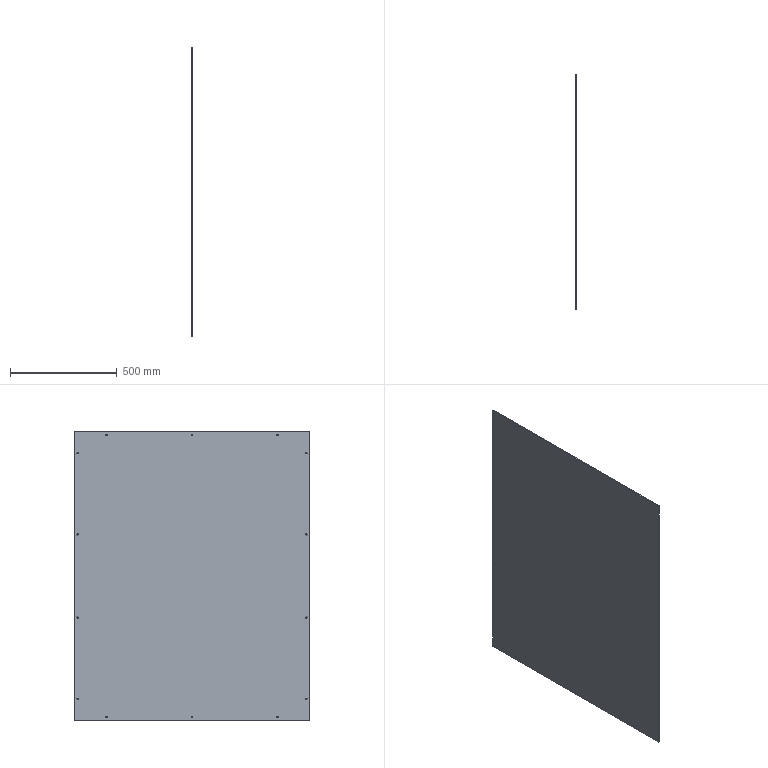Part | STEP file | 08-06 Guard top cover plate | 1 solid | 34 faces | box 5 x 1100 x 1350 mm | volume 7422677 mm3 | cylinder 28 | plane 6 | commonest cylinder face diameters 6.5 x28